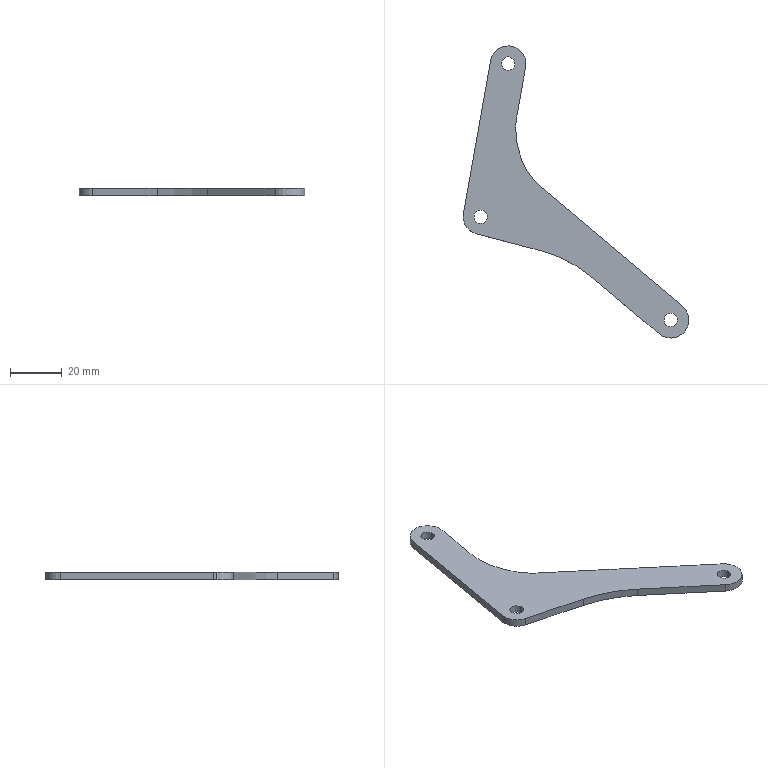Part | SolidWorks | features BaseBody 1 | 1 solid | 20 faces | box 87.081 x 112.72 x 3 mm | volume 7302 mm3 | cylinder 13 | plane 7 | commonest cylinder face diameters 5.2 x6 13.58 x2 62.282 x2 13.715 x1 14 x1 100 x1
STEP:
#1=CARTESIAN_POINT('',(62.068,74.152,3.));
#2=VERTEX_POINT('',#1);
#3=CARTESIAN_POINT('',(56.868,74.152,3.));
#4=VERTEX_POINT('',#3);
#5=CARTESIAN_POINT('',(59.468,74.152,3.));
#6=DIRECTION('',(0.,0.,-1.));
#7=DIRECTION('',(-1.,0.,0.));
#8=AXIS2_PLACEMENT_3D('',#5,#6,#7);
#9=CIRCLE('',#8,2.6);
#10=EDGE_CURVE('',#2,#4,#9,.T.);
#11=ORIENTED_EDGE('',*,*,#10,.F.);
#12=CARTESIAN_POINT('',(62.068,74.152,0.));
#13=VERTEX_POINT('',#12);
#14=CARTESIAN_POINT('',(62.068,74.152,3.));
#15=DIRECTION('',(0.,0.,-1.));
#16=VECTOR('',#15,1000.);
#17=LINE('',#14,#16);
#18=EDGE_CURVE('',#2,#13,#17,.T.);
#19=ORIENTED_EDGE('',*,*,#18,.T.);
#20=CARTESIAN_POINT('',(56.868,74.152,0.));
#21=VERTEX_POINT('',#20);
#22=CARTESIAN_POINT('',(59.468,74.152,0.));
#23=DIRECTION('',(0.,0.,1.));
#24=DIRECTION('',(-1.,0.,0.));
#25=AXIS2_PLACEMENT_3D('',#22,#23,#24);
#26=CIRCLE('',#25,2.6);
#27=EDGE_CURVE('',#21,#13,#26,.T.);
#28=ORIENTED_EDGE('',*,*,#27,.F.);
#29=CARTESIAN_POINT('',(56.868,74.152,3.));
#30=DIRECTION('',(0.,0.,-1.));
#31=VECTOR('',#30,1000.);
#32=LINE('',#29,#31);
#33=EDGE_CURVE('',#4,#21,#32,.T.);
#34=ORIENTED_EDGE('',*,*,#33,.F.);
#35=EDGE_LOOP('',(#11,#19,#28,#34));
#36=FACE_OUTER_BOUND('',#35,.T.);
#37=CARTESIAN_POINT('',(59.468,74.152,3.));
#38=DIRECTION('',(0.,0.,-1.));
#39=DIRECTION('',(-1.,0.,0.));
#40=AXIS2_PLACEMENT_3D('',#37,#38,#39);
#41=CYLINDRICAL_SURFACE('',#40,2.6);
#42=ADVANCED_FACE('',(#36),#41,.F.);
#43=CARTESIAN_POINT('',(62.402,48.808,3.));
#44=VERTEX_POINT('',#43);
#45=CARTESIAN_POINT('',(63.076,55.251,3.));
#46=VERTEX_POINT('',#45);
#47=CARTESIAN_POINT('',(93.543,48.808,3.));
#48=DIRECTION('',(0.,0.,-1.));
#49=DIRECTION('',(-1.,0.,0.));
#50=AXIS2_PLACEMENT_3D('',#47,#48,#49);
#51=CIRCLE('',#50,31.141);
#52=EDGE_CURVE('',#44,#46,#51,.T.);
#53=ORIENTED_EDGE('',*,*,#52,.F.);
#54=CARTESIAN_POINT('',(62.402,48.808,0.));
#55=VERTEX_POINT('',#54);
#56=CARTESIAN_POINT('',(62.402,48.808,3.));
#57=DIRECTION('',(0.,0.,-1.));
#58=VECTOR('',#57,1000.);
#59=LINE('',#56,#58);
#60=EDGE_CURVE('',#44,#55,#59,.T.);
#61=ORIENTED_EDGE('',*,*,#60,.T.);
#62=CARTESIAN_POINT('',(63.076,55.251,0.));
#63=VERTEX_POINT('',#62);
#64=CARTESIAN_POINT('',(93.543,48.808,0.));
#65=DIRECTION('',(0.,0.,1.));
#66=DIRECTION('',(-1.,0.,0.));
#67=AXIS2_PLACEMENT_3D('',#64,#65,#66);
#68=CIRCLE('',#67,31.141);
#69=EDGE_CURVE('',#63,#55,#68,.T.);
#70=ORIENTED_EDGE('',*,*,#69,.F.);
#71=CARTESIAN_POINT('',(63.076,55.251,3.));
#72=DIRECTION('',(0.,0.,-1.));
#73=VECTOR('',#72,1000.);
#74=LINE('',#71,#73);
#75=EDGE_CURVE('',#46,#63,#74,.T.);
#76=ORIENTED_EDGE('',*,*,#75,.F.);
#77=EDGE_LOOP('',(#53,#61,#70,#76));
#78=FACE_OUTER_BOUND('',#77,.T.);
#79=CARTESIAN_POINT('',(93.543,48.808,3.));
#80=DIRECTION('',(0.,0.,-1.));
#81=DIRECTION('',(-1.,0.,0.));
#82=AXIS2_PLACEMENT_3D('',#79,#80,#81);
#83=CYLINDRICAL_SURFACE('',#82,31.141);
#84=ADVANCED_FACE('',(#78),#83,.F.);
#85=CARTESIAN_POINT('',(42.12,15.088,3.));
#86=VERTEX_POINT('',#85);
#87=CARTESIAN_POINT('',(47.182,8.522,3.));
#88=VERTEX_POINT('',#87);
#89=CARTESIAN_POINT('',(48.91,15.088,3.));
#90=DIRECTION('',(0.,0.,1.));
#91=DIRECTION('',(-1.,0.,0.));
#92=AXIS2_PLACEMENT_3D('',#89,#90,#91);
#93=CIRCLE('',#92,6.79);
#94=EDGE_CURVE('',#86,#88,#93,.T.);
#95=ORIENTED_EDGE('',*,*,#94,.F.);
#96=CARTESIAN_POINT('',(42.12,15.088,0.));
#97=VERTEX_POINT('',#96);
#98=CARTESIAN_POINT('',(42.12,15.088,3.));
#99=DIRECTION('',(0.,0.,-1.));
#100=VECTOR('',#99,1000.);
#101=LINE('',#98,#100);
#102=EDGE_CURVE('',#86,#97,#101,.T.);
#103=ORIENTED_EDGE('',*,*,#102,.T.);
#104=CARTESIAN_POINT('',(47.182,8.522,0.));
#105=VERTEX_POINT('',#104);
#106=CARTESIAN_POINT('',(48.91,15.088,0.));
#107=DIRECTION('',(0.,0.,1.));
#108=DIRECTION('',(-1.,0.,0.));
#109=AXIS2_PLACEMENT_3D('',#106,#107,#108);
#110=CIRCLE('',#109,6.79);
#111=EDGE_CURVE('',#97,#105,#110,.T.);
#112=ORIENTED_EDGE('',*,*,#111,.T.);
#113=CARTESIAN_POINT('',(47.182,8.522,3.));
#114=DIRECTION('',(0.,0.,1.));
#115=VECTOR('',#114,1000.);
#116=LINE('',#113,#115);
#117=EDGE_CURVE('',#105,#88,#116,.T.);
#118=ORIENTED_EDGE('',*,*,#117,.T.);
#119=EDGE_LOOP('',(#95,#103,#112,#118));
#120=FACE_OUTER_BOUND('',#119,.T.);
#121=CARTESIAN_POINT('',(48.91,15.088,3.));
#122=DIRECTION('',(0.,0.,-1.));
#123=DIRECTION('',(-1.,0.,0.));
#124=AXIS2_PLACEMENT_3D('',#121,#122,#123);
#125=CYLINDRICAL_SURFACE('',#124,6.79);
#126=ADVANCED_FACE('',(#120),#125,.T.);
#127=CARTESIAN_POINT('',(124.801,-24.711,3.));
#128=VERTEX_POINT('',#127);
#129=CARTESIAN_POINT('',(119.601,-24.711,3.));
#130=VERTEX_POINT('',#129);
#131=CARTESIAN_POINT('',(122.201,-24.711,3.));
#132=DIRECTION('',(0.,0.,-1.));
#133=DIRECTION('',(-1.,0.,0.));
#134=AXIS2_PLACEMENT_3D('',#131,#132,#133);
#135=CIRCLE('',#134,2.6);
#136=EDGE_CURVE('',#128,#130,#135,.T.);
#137=ORIENTED_EDGE('',*,*,#136,.F.);
#138=CARTESIAN_POINT('',(124.801,-24.711,0.));
#139=VERTEX_POINT('',#138);
#140=CARTESIAN_POINT('',(124.801,-24.711,3.));
#141=DIRECTION('',(0.,0.,-1.));
#142=VECTOR('',#141,1000.);
#143=LINE('',#140,#142);
#144=EDGE_CURVE('',#128,#139,#143,.T.);
#145=ORIENTED_EDGE('',*,*,#144,.T.);
#146=CARTESIAN_POINT('',(119.601,-24.711,0.));
#147=VERTEX_POINT('',#146);
#148=CARTESIAN_POINT('',(122.201,-24.711,0.));
#149=DIRECTION('',(0.,0.,1.));
#150=DIRECTION('',(-1.,0.,0.));
#151=AXIS2_PLACEMENT_3D('',#148,#149,#150);
#152=CIRCLE('',#151,2.6);
#153=EDGE_CURVE('',#147,#139,#152,.T.);
#154=ORIENTED_EDGE('',*,*,#153,.F.);
#155=CARTESIAN_POINT('',(119.601,-24.711,3.));
#156=DIRECTION('',(0.,0.,-1.));
#157=VECTOR('',#156,1000.);
#158=LINE('',#155,#157);
#159=EDGE_CURVE('',#130,#147,#158,.T.);
#160=ORIENTED_EDGE('',*,*,#159,.F.);
#161=EDGE_LOOP('',(#137,#145,#154,#160));
#162=FACE_OUTER_BOUND('',#161,.T.);
#163=CARTESIAN_POINT('',(122.201,-24.711,3.));
#164=DIRECTION('',(0.,0.,-1.));
#165=DIRECTION('',(-1.,0.,0.));
#166=AXIS2_PLACEMENT_3D('',#163,#164,#165);
#167=CYLINDRICAL_SURFACE('',#166,2.6);
#168=ADVANCED_FACE('',(#162),#167,.F.);
#169=CARTESIAN_POINT('',(51.51,15.088,3.));
#170=VERTEX_POINT('',#169);
#171=CARTESIAN_POINT('',(46.31,15.088,3.));
#172=VERTEX_POINT('',#171);
#173=CARTESIAN_POINT('',(48.91,15.088,3.));
#174=DIRECTION('',(0.,0.,-1.));
#175=DIRECTION('',(-1.,0.,0.));
#176=AXIS2_PLACEMENT_3D('',#173,#174,#175);
#177=CIRCLE('',#176,2.6);
#178=EDGE_CURVE('',#170,#172,#177,.T.);
#179=ORIENTED_EDGE('',*,*,#178,.F.);
#180=CARTESIAN_POINT('',(51.51,15.088,0.));
#181=VERTEX_POINT('',#180);
#182=CARTESIAN_POINT('',(51.51,15.088,3.));
#183=DIRECTION('',(0.,0.,-1.));
#184=VECTOR('',#183,1000.);
#185=LINE('',#182,#184);
#186=EDGE_CURVE('',#170,#181,#185,.T.);
#187=ORIENTED_EDGE('',*,*,#186,.T.);
#188=CARTESIAN_POINT('',(46.31,15.088,0.));
#189=VERTEX_POINT('',#188);
#190=CARTESIAN_POINT('',(48.91,15.088,0.));
#191=DIRECTION('',(0.,0.,1.));
#192=DIRECTION('',(-1.,0.,0.));
#193=AXIS2_PLACEMENT_3D('',#190,#191,#192);
#194=CIRCLE('',#193,2.6);
#195=EDGE_CURVE('',#189,#181,#194,.T.);
#196=ORIENTED_EDGE('',*,*,#195,.F.);
#197=CARTESIAN_POINT('',(46.31,15.088,3.));
#198=DIRECTION('',(0.,0.,-1.));
#199=VECTOR('',#198,1000.);
#200=LINE('',#197,#199);
#201=EDGE_CURVE('',#172,#189,#200,.T.);
#202=ORIENTED_EDGE('',*,*,#201,.F.);
#203=EDGE_LOOP('',(#179,#187,#196,#202));
#204=FACE_OUTER_BOUND('',#203,.T.);
#205=CARTESIAN_POINT('',(48.91,15.088,3.));
#206=DIRECTION('',(0.,0.,-1.));
#207=DIRECTION('',(-1.,0.,0.));
#208=AXIS2_PLACEMENT_3D('',#205,#206,#207);
#209=CYLINDRICAL_SURFACE('',#208,2.6);
#210=ADVANCED_FACE('',(#204),#209,.F.);
#211=CARTESIAN_POINT('',(59.468,74.152,3.));
#212=DIRECTION('',(0.,0.,-1.));
#213=DIRECTION('',(-1.,0.,0.));
#214=AXIS2_PLACEMENT_3D('',#211,#212,#213);
#215=CIRCLE('',#214,2.6);
#216=EDGE_CURVE('',#4,#2,#215,.T.);
#217=ORIENTED_EDGE('',*,*,#216,.T.);
#218=ORIENTED_EDGE('',*,*,#10,.T.);
#219=EDGE_LOOP('',(#217,#218));
#220=FACE_BOUND('',#219,.T.);
#221=CARTESIAN_POINT('',(70.256,28.133,3.));
#222=VERTEX_POINT('',#221);
#223=CARTESIAN_POINT('',(93.543,48.808,3.));
#224=DIRECTION('',(0.,0.,-1.));
#225=DIRECTION('',(-1.,0.,0.));
#226=AXIS2_PLACEMENT_3D('',#223,#224,#225);
#227=CIRCLE('',#226,31.141);
#228=EDGE_CURVE('',#222,#44,#227,.T.);
#229=ORIENTED_EDGE('',*,*,#228,.T.);
#230=ORIENTED_EDGE('',*,*,#52,.T.);
#231=CARTESIAN_POINT('',(66.219,72.953,3.));
#232=VERTEX_POINT('',#231);
#233=CARTESIAN_POINT('',(63.076,55.251,3.));
#234=DIRECTION('',(0.1749,0.9846,0.));
#235=VECTOR('',#234,1000.);
#236=LINE('',#233,#235);
#237=EDGE_CURVE('',#46,#232,#236,.T.);
#238=ORIENTED_EDGE('',*,*,#237,.T.);
#239=CARTESIAN_POINT('',(52.716,75.351,3.));
#240=VERTEX_POINT('',#239);
#241=CARTESIAN_POINT('',(59.468,74.152,3.));
#242=DIRECTION('',(0.,0.,1.));
#243=DIRECTION('',(-1.,0.,0.));
#244=AXIS2_PLACEMENT_3D('',#241,#242,#243);
#245=CIRCLE('',#244,6.857);
#246=EDGE_CURVE('',#232,#240,#245,.T.);
#247=ORIENTED_EDGE('',*,*,#246,.T.);
#248=CARTESIAN_POINT('',(42.225,16.276,3.));
#249=VERTEX_POINT('',#248);
#250=CARTESIAN_POINT('',(52.716,75.351,3.));
#251=DIRECTION('',(-0.1749,-0.9846,0.));
#252=VECTOR('',#251,1000.);
#253=LINE('',#250,#252);
#254=EDGE_CURVE('',#240,#249,#253,.T.);
#255=ORIENTED_EDGE('',*,*,#254,.T.);
#256=CARTESIAN_POINT('',(48.91,15.088,3.));
#257=DIRECTION('',(0.,0.,1.));
#258=DIRECTION('',(-1.,0.,0.));
#259=AXIS2_PLACEMENT_3D('',#256,#257,#258);
#260=CIRCLE('',#259,6.79);
#261=EDGE_CURVE('',#249,#86,#260,.T.);
#262=ORIENTED_EDGE('',*,*,#261,.T.);
#263=ORIENTED_EDGE('',*,*,#94,.T.);
#264=CARTESIAN_POINT('',(72.182,1.941,3.));
#265=VERTEX_POINT('',#264);
#266=CARTESIAN_POINT('',(47.182,8.522,3.));
#267=DIRECTION('',(0.9671,-0.2546,0.));
#268=VECTOR('',#267,1000.);
#269=LINE('',#266,#268);
#270=EDGE_CURVE('',#88,#265,#269,.T.);
#271=ORIENTED_EDGE('',*,*,#270,.T.);
#272=CARTESIAN_POINT('',(91.639,-8.149,3.));
#273=VERTEX_POINT('',#272);
#274=CARTESIAN_POINT('',(59.453,-46.412,3.));
#275=DIRECTION('',(0.,0.,-1.));
#276=DIRECTION('',(-1.,0.,0.));
#277=AXIS2_PLACEMENT_3D('',#274,#275,#276);
#278=CIRCLE('',#277,50.);
#279=EDGE_CURVE('',#265,#273,#278,.T.);
#280=ORIENTED_EDGE('',*,*,#279,.T.);
#281=CARTESIAN_POINT('',(117.695,-30.067,3.));
#282=VERTEX_POINT('',#281);
#283=CARTESIAN_POINT('',(91.639,-8.149,3.));
#284=DIRECTION('',(0.7653,-0.6437,0.));
#285=VECTOR('',#284,1000.);
#286=LINE('',#283,#285);
#287=EDGE_CURVE('',#273,#282,#286,.T.);
#288=ORIENTED_EDGE('',*,*,#287,.T.);
#289=CARTESIAN_POINT('',(126.707,-19.354,3.));
#290=VERTEX_POINT('',#289);
#291=CARTESIAN_POINT('',(122.201,-24.711,3.));
#292=DIRECTION('',(0.,0.,1.));
#293=DIRECTION('',(-1.,0.,0.));
#294=AXIS2_PLACEMENT_3D('',#291,#292,#293);
#295=CIRCLE('',#294,7.);
#296=EDGE_CURVE('',#282,#290,#295,.T.);
#297=ORIENTED_EDGE('',*,*,#296,.T.);
#298=CARTESIAN_POINT('',(126.707,-19.354,3.));
#299=DIRECTION('',(-0.7653,0.6437,0.));
#300=VECTOR('',#299,1000.);
#301=LINE('',#298,#300);
#302=EDGE_CURVE('',#290,#222,#301,.T.);
#303=ORIENTED_EDGE('',*,*,#302,.T.);
#304=EDGE_LOOP('',(#229,#230,#238,#247,#255,#262,#263,#271,#280,#288,#297,#303));
#305=FACE_OUTER_BOUND('',#304,.T.);
#306=CARTESIAN_POINT('',(122.201,-24.711,3.));
#307=DIRECTION('',(0.,0.,-1.));
#308=DIRECTION('',(-1.,0.,0.));
#309=AXIS2_PLACEMENT_3D('',#306,#307,#308);
#310=CIRCLE('',#309,2.6);
#311=EDGE_CURVE('',#130,#128,#310,.T.);
#312=ORIENTED_EDGE('',*,*,#311,.T.);
#313=ORIENTED_EDGE('',*,*,#136,.T.);
#314=EDGE_LOOP('',(#312,#313));
#315=FACE_BOUND('',#314,.T.);
#316=CARTESIAN_POINT('',(48.91,15.088,3.));
#317=DIRECTION('',(0.,0.,-1.));
#318=DIRECTION('',(-1.,0.,0.));
#319=AXIS2_PLACEMENT_3D('',#316,#317,#318);
#320=CIRCLE('',#319,2.6);
#321=EDGE_CURVE('',#172,#170,#320,.T.);
#322=ORIENTED_EDGE('',*,*,#321,.T.);
#323=ORIENTED_EDGE('',*,*,#178,.T.);
#324=EDGE_LOOP('',(#322,#323));
#325=FACE_BOUND('',#324,.T.);
#326=CARTESIAN_POINT('',(48.91,15.088,3.));
#327=DIRECTION('',(0.,0.,1.));
#328=DIRECTION('',(1.,0.,0.));
#329=AXIS2_PLACEMENT_3D('',#326,#327,#328);
#330=PLANE('',#329);
#331=ADVANCED_FACE('',(#220,#305,#315,#325),#330,.T.);
#332=ORIENTED_EDGE('',*,*,#18,.F.);
#333=ORIENTED_EDGE('',*,*,#216,.F.);
#334=ORIENTED_EDGE('',*,*,#33,.T.);
#335=CARTESIAN_POINT('',(59.468,74.152,0.));
#336=DIRECTION('',(0.,0.,1.));
#337=DIRECTION('',(-1.,0.,0.));
#338=AXIS2_PLACEMENT_3D('',#335,#336,#337);
#339=CIRCLE('',#338,2.6);
#340=EDGE_CURVE('',#13,#21,#339,.T.);
#341=ORIENTED_EDGE('',*,*,#340,.F.);
#342=EDGE_LOOP('',(#332,#333,#334,#341));
#343=FACE_OUTER_BOUND('',#342,.T.);
#344=CARTESIAN_POINT('',(59.468,74.152,3.));
#345=DIRECTION('',(0.,0.,-1.));
#346=DIRECTION('',(-1.,0.,0.));
#347=AXIS2_PLACEMENT_3D('',#344,#345,#346);
#348=CYLINDRICAL_SURFACE('',#347,2.6);
#349=ADVANCED_FACE('',(#343),#348,.F.);
#350=ORIENTED_EDGE('',*,*,#60,.F.);
#351=ORIENTED_EDGE('',*,*,#228,.F.);
#352=CARTESIAN_POINT('',(70.256,28.133,0.));
#353=VERTEX_POINT('',#352);
#354=CARTESIAN_POINT('',(70.256,28.133,3.));
#355=DIRECTION('',(0.,0.,1.));
#356=VECTOR('',#355,1000.);
#357=LINE('',#354,#356);
#358=EDGE_CURVE('',#353,#222,#357,.T.);
#359=ORIENTED_EDGE('',*,*,#358,.F.);
#360=CARTESIAN_POINT('',(93.543,48.808,0.));
#361=DIRECTION('',(0.,0.,1.));
#362=DIRECTION('',(-1.,0.,0.));
#363=AXIS2_PLACEMENT_3D('',#360,#361,#362);
#364=CIRCLE('',#363,31.141);
#365=EDGE_CURVE('',#55,#353,#364,.T.);
#366=ORIENTED_EDGE('',*,*,#365,.F.);
#367=EDGE_LOOP('',(#350,#351,#359,#366));
#368=FACE_OUTER_BOUND('',#367,.T.);
#369=CARTESIAN_POINT('',(93.543,48.808,3.));
#370=DIRECTION('',(0.,0.,-1.));
#371=DIRECTION('',(-1.,0.,0.));
#372=AXIS2_PLACEMENT_3D('',#369,#370,#371);
#373=CYLINDRICAL_SURFACE('',#372,31.141);
#374=ADVANCED_FACE('',(#368),#373,.F.);
#375=ORIENTED_EDGE('',*,*,#302,.F.);
#376=CARTESIAN_POINT('',(126.707,-19.354,0.));
#377=VERTEX_POINT('',#376);
#378=CARTESIAN_POINT('',(126.707,-19.354,3.));
#379=DIRECTION('',(0.,0.,1.));
#380=VECTOR('',#379,1000.);
#381=LINE('',#378,#380);
#382=EDGE_CURVE('',#377,#290,#381,.T.);
#383=ORIENTED_EDGE('',*,*,#382,.F.);
#384=CARTESIAN_POINT('',(70.256,28.133,0.));
#385=DIRECTION('',(0.7653,-0.6437,0.));
#386=VECTOR('',#385,1000.);
#387=LINE('',#384,#386);
#388=EDGE_CURVE('',#353,#377,#387,.T.);
#389=ORIENTED_EDGE('',*,*,#388,.F.);
#390=ORIENTED_EDGE('',*,*,#358,.T.);
#391=EDGE_LOOP('',(#375,#383,#389,#390));
#392=FACE_OUTER_BOUND('',#391,.T.);
#393=CARTESIAN_POINT('',(70.256,28.133,3.));
#394=DIRECTION('',(-0.6437,-0.7653,0.));
#395=DIRECTION('',(0.7653,-0.6437,0.));
#396=AXIS2_PLACEMENT_3D('',#393,#394,#395);
#397=PLANE('',#396);
#398=ADVANCED_FACE('',(#392),#397,.F.);
#399=CARTESIAN_POINT('',(117.695,-30.067,0.));
#400=VERTEX_POINT('',#399);
#401=CARTESIAN_POINT('',(122.201,-24.711,0.));
#402=DIRECTION('',(0.,0.,1.));
#403=DIRECTION('',(-1.,0.,0.));
#404=AXIS2_PLACEMENT_3D('',#401,#402,#403);
#405=CIRCLE('',#404,7.);
#406=EDGE_CURVE('',#400,#377,#405,.T.);
#407=ORIENTED_EDGE('',*,*,#406,.T.);
#408=ORIENTED_EDGE('',*,*,#382,.T.);
#409=ORIENTED_EDGE('',*,*,#296,.F.);
#410=CARTESIAN_POINT('',(117.695,-30.067,3.));
#411=DIRECTION('',(0.,0.,-1.));
#412=VECTOR('',#411,1000.);
#413=LINE('',#410,#412);
#414=EDGE_CURVE('',#282,#400,#413,.T.);
#415=ORIENTED_EDGE('',*,*,#414,.T.);
#416=EDGE_LOOP('',(#407,#408,#409,#415));
#417=FACE_OUTER_BOUND('',#416,.T.);
#418=CARTESIAN_POINT('',(122.201,-24.711,3.));
#419=DIRECTION('',(0.,0.,-1.));
#420=DIRECTION('',(-1.,0.,0.));
#421=AXIS2_PLACEMENT_3D('',#418,#419,#420);
#422=CYLINDRICAL_SURFACE('',#421,7.);
#423=ADVANCED_FACE('',(#417),#422,.T.);
#424=ORIENTED_EDGE('',*,*,#287,.F.);
#425=CARTESIAN_POINT('',(91.639,-8.149,0.));
#426=VERTEX_POINT('',#425);
#427=CARTESIAN_POINT('',(91.639,-8.149,3.));
#428=DIRECTION('',(0.,0.,1.));
#429=VECTOR('',#428,1000.);
#430=LINE('',#427,#429);
#431=EDGE_CURVE('',#426,#273,#430,.T.);
#432=ORIENTED_EDGE('',*,*,#431,.F.);
#433=CARTESIAN_POINT('',(117.695,-30.067,0.));
#434=DIRECTION('',(-0.7653,0.6437,0.));
#435=VECTOR('',#434,1000.);
#436=LINE('',#433,#435);
#437=EDGE_CURVE('',#400,#426,#436,.T.);
#438=ORIENTED_EDGE('',*,*,#437,.F.);
#439=ORIENTED_EDGE('',*,*,#414,.F.);
#440=EDGE_LOOP('',(#424,#432,#438,#439));
#441=FACE_OUTER_BOUND('',#440,.T.);
#442=CARTESIAN_POINT('',(117.695,-30.067,3.));
#443=DIRECTION('',(0.6437,0.7653,0.));
#444=DIRECTION('',(-0.7653,0.6437,0.));
#445=AXIS2_PLACEMENT_3D('',#442,#443,#444);
#446=PLANE('',#445);
#447=ADVANCED_FACE('',(#441),#446,.F.);
#448=ORIENTED_EDGE('',*,*,#279,.F.);
#449=CARTESIAN_POINT('',(72.182,1.941,0.));
#450=VERTEX_POINT('',#449);
#451=CARTESIAN_POINT('',(72.182,1.941,3.));
#452=DIRECTION('',(0.,0.,1.));
#453=VECTOR('',#452,1000.);
#454=LINE('',#451,#453);
#455=EDGE_CURVE('',#450,#265,#454,.T.);
#456=ORIENTED_EDGE('',*,*,#455,.F.);
#457=CARTESIAN_POINT('',(59.453,-46.412,0.));
#458=DIRECTION('',(0.,0.,1.));
#459=DIRECTION('',(-1.,0.,0.));
#460=AXIS2_PLACEMENT_3D('',#457,#458,#459);
#461=CIRCLE('',#460,50.);
#462=EDGE_CURVE('',#426,#450,#461,.T.);
#463=ORIENTED_EDGE('',*,*,#462,.F.);
#464=ORIENTED_EDGE('',*,*,#431,.T.);
#465=EDGE_LOOP('',(#448,#456,#463,#464));
#466=FACE_OUTER_BOUND('',#465,.T.);
#467=CARTESIAN_POINT('',(59.453,-46.412,3.));
#468=DIRECTION('',(0.,0.,-1.));
#469=DIRECTION('',(-1.,0.,0.));
#470=AXIS2_PLACEMENT_3D('',#467,#468,#469);
#471=CYLINDRICAL_SURFACE('',#470,50.);
#472=ADVANCED_FACE('',(#466),#471,.F.);
#473=ORIENTED_EDGE('',*,*,#270,.F.);
#474=ORIENTED_EDGE('',*,*,#117,.F.);
#475=CARTESIAN_POINT('',(72.182,1.941,0.));
#476=DIRECTION('',(-0.9671,0.2546,0.));
#477=VECTOR('',#476,1000.);
#478=LINE('',#475,#477);
#479=EDGE_CURVE('',#450,#105,#478,.T.);
#480=ORIENTED_EDGE('',*,*,#479,.F.);
#481=ORIENTED_EDGE('',*,*,#455,.T.);
#482=EDGE_LOOP('',(#473,#474,#480,#481));
#483=FACE_OUTER_BOUND('',#482,.T.);
#484=CARTESIAN_POINT('',(72.182,1.941,3.));
#485=DIRECTION('',(0.2546,0.9671,0.));
#486=DIRECTION('',(-0.9671,0.2546,0.));
#487=AXIS2_PLACEMENT_3D('',#484,#485,#486);
#488=PLANE('',#487);
#489=ADVANCED_FACE('',(#483),#488,.F.);
#490=ORIENTED_EDGE('',*,*,#102,.F.);
#491=ORIENTED_EDGE('',*,*,#261,.F.);
#492=CARTESIAN_POINT('',(42.225,16.276,0.));
#493=VERTEX_POINT('',#492);
#494=CARTESIAN_POINT('',(42.225,16.276,3.));
#495=DIRECTION('',(0.,0.,-1.));
#496=VECTOR('',#495,1000.);
#497=LINE('',#494,#496);
#498=EDGE_CURVE('',#249,#493,#497,.T.);
#499=ORIENTED_EDGE('',*,*,#498,.T.);
#500=CARTESIAN_POINT('',(48.91,15.088,0.));
#501=DIRECTION('',(0.,0.,1.));
#502=DIRECTION('',(-1.,0.,0.));
#503=AXIS2_PLACEMENT_3D('',#500,#501,#502);
#504=CIRCLE('',#503,6.79);
#505=EDGE_CURVE('',#493,#97,#504,.T.);
#506=ORIENTED_EDGE('',*,*,#505,.T.);
#507=EDGE_LOOP('',(#490,#491,#499,#506));
#508=FACE_OUTER_BOUND('',#507,.T.);
#509=CARTESIAN_POINT('',(48.91,15.088,3.));
#510=DIRECTION('',(0.,0.,-1.));
#511=DIRECTION('',(-1.,0.,0.));
#512=AXIS2_PLACEMENT_3D('',#509,#510,#511);
#513=CYLINDRICAL_SURFACE('',#512,6.79);
#514=ADVANCED_FACE('',(#508),#513,.T.);
#515=ORIENTED_EDGE('',*,*,#254,.F.);
#516=CARTESIAN_POINT('',(52.716,75.351,0.));
#517=VERTEX_POINT('',#516);
#518=CARTESIAN_POINT('',(52.716,75.351,3.));
#519=DIRECTION('',(0.,0.,1.));
#520=VECTOR('',#519,1000.);
#521=LINE('',#518,#520);
#522=EDGE_CURVE('',#517,#240,#521,.T.);
#523=ORIENTED_EDGE('',*,*,#522,.F.);
#524=CARTESIAN_POINT('',(46.025,37.673,0.));
#525=DIRECTION('',(0.1749,0.9846,0.));
#526=VECTOR('',#525,1000.);
#527=LINE('',#524,#526);
#528=EDGE_CURVE('',#493,#517,#527,.T.);
#529=ORIENTED_EDGE('',*,*,#528,.F.);
#530=ORIENTED_EDGE('',*,*,#498,.F.);
#531=EDGE_LOOP('',(#515,#523,#529,#530));
#532=FACE_OUTER_BOUND('',#531,.T.);
#533=CARTESIAN_POINT('',(46.025,37.673,3.));
#534=DIRECTION('',(0.9846,-0.1749,0.));
#535=DIRECTION('',(0.1749,0.9846,0.));
#536=AXIS2_PLACEMENT_3D('',#533,#534,#535);
#537=PLANE('',#536);
#538=ADVANCED_FACE('',(#532),#537,.F.);
#539=CARTESIAN_POINT('',(66.219,72.953,0.));
#540=VERTEX_POINT('',#539);
#541=CARTESIAN_POINT('',(59.468,74.152,0.));
#542=DIRECTION('',(0.,0.,1.));
#543=DIRECTION('',(-1.,0.,0.));
#544=AXIS2_PLACEMENT_3D('',#541,#542,#543);
#545=CIRCLE('',#544,6.857);
#546=EDGE_CURVE('',#540,#517,#545,.T.);
#547=ORIENTED_EDGE('',*,*,#546,.T.);
#548=ORIENTED_EDGE('',*,*,#522,.T.);
#549=ORIENTED_EDGE('',*,*,#246,.F.);
#550=CARTESIAN_POINT('',(66.219,72.953,3.));
#551=DIRECTION('',(0.,0.,-1.));
#552=VECTOR('',#551,1000.);
#553=LINE('',#550,#552);
#554=EDGE_CURVE('',#232,#540,#553,.T.);
#555=ORIENTED_EDGE('',*,*,#554,.T.);
#556=EDGE_LOOP('',(#547,#548,#549,#555));
#557=FACE_OUTER_BOUND('',#556,.T.);
#558=CARTESIAN_POINT('',(59.468,74.152,3.));
#559=DIRECTION('',(0.,0.,-1.));
#560=DIRECTION('',(-1.,0.,0.));
#561=AXIS2_PLACEMENT_3D('',#558,#559,#560);
#562=CYLINDRICAL_SURFACE('',#561,6.857);
#563=ADVANCED_FACE('',(#557),#562,.T.);
#564=ORIENTED_EDGE('',*,*,#237,.F.);
#565=ORIENTED_EDGE('',*,*,#75,.T.);
#566=CARTESIAN_POINT('',(66.219,72.953,0.));
#567=DIRECTION('',(-0.1749,-0.9846,0.));
#568=VECTOR('',#567,1000.);
#569=LINE('',#566,#568);
#570=EDGE_CURVE('',#540,#63,#569,.T.);
#571=ORIENTED_EDGE('',*,*,#570,.F.);
#572=ORIENTED_EDGE('',*,*,#554,.F.);
#573=EDGE_LOOP('',(#564,#565,#571,#572));
#574=FACE_OUTER_BOUND('',#573,.T.);
#575=CARTESIAN_POINT('',(66.219,72.953,3.));
#576=DIRECTION('',(-0.9846,0.1749,0.));
#577=DIRECTION('',(-0.1749,-0.9846,0.));
#578=AXIS2_PLACEMENT_3D('',#575,#576,#577);
#579=PLANE('',#578);
#580=ADVANCED_FACE('',(#574),#579,.F.);
#581=ORIENTED_EDGE('',*,*,#144,.F.);
#582=ORIENTED_EDGE('',*,*,#311,.F.);
#583=ORIENTED_EDGE('',*,*,#159,.T.);
#584=CARTESIAN_POINT('',(122.201,-24.711,0.));
#585=DIRECTION('',(0.,0.,1.));
#586=DIRECTION('',(-1.,0.,0.));
#587=AXIS2_PLACEMENT_3D('',#584,#585,#586);
#588=CIRCLE('',#587,2.6);
#589=EDGE_CURVE('',#139,#147,#588,.T.);
#590=ORIENTED_EDGE('',*,*,#589,.F.);
#591=EDGE_LOOP('',(#581,#582,#583,#590));
#592=FACE_OUTER_BOUND('',#591,.T.);
#593=CARTESIAN_POINT('',(122.201,-24.711,3.));
#594=DIRECTION('',(0.,0.,-1.));
#595=DIRECTION('',(-1.,0.,0.));
#596=AXIS2_PLACEMENT_3D('',#593,#594,#595);
#597=CYLINDRICAL_SURFACE('',#596,2.6);
#598=ADVANCED_FACE('',(#592),#597,.F.);
#599=ORIENTED_EDGE('',*,*,#186,.F.);
#600=ORIENTED_EDGE('',*,*,#321,.F.);
#601=ORIENTED_EDGE('',*,*,#201,.T.);
#602=CARTESIAN_POINT('',(48.91,15.088,0.));
#603=DIRECTION('',(0.,0.,1.));
#604=DIRECTION('',(-1.,0.,0.));
#605=AXIS2_PLACEMENT_3D('',#602,#603,#604);
#606=CIRCLE('',#605,2.6);
#607=EDGE_CURVE('',#181,#189,#606,.T.);
#608=ORIENTED_EDGE('',*,*,#607,.F.);
#609=EDGE_LOOP('',(#599,#600,#601,#608));
#610=FACE_OUTER_BOUND('',#609,.T.);
#611=CARTESIAN_POINT('',(48.91,15.088,3.));
#612=DIRECTION('',(0.,0.,-1.));
#613=DIRECTION('',(-1.,0.,0.));
#614=AXIS2_PLACEMENT_3D('',#611,#612,#613);
#615=CYLINDRICAL_SURFACE('',#614,2.6);
#616=ADVANCED_FACE('',(#610),#615,.F.);
#617=ORIENTED_EDGE('',*,*,#546,.F.);
#618=ORIENTED_EDGE('',*,*,#570,.T.);
#619=ORIENTED_EDGE('',*,*,#69,.T.);
#620=ORIENTED_EDGE('',*,*,#365,.T.);
#621=ORIENTED_EDGE('',*,*,#388,.T.);
#622=ORIENTED_EDGE('',*,*,#406,.F.);
#623=ORIENTED_EDGE('',*,*,#437,.T.);
#624=ORIENTED_EDGE('',*,*,#462,.T.);
#625=ORIENTED_EDGE('',*,*,#479,.T.);
#626=ORIENTED_EDGE('',*,*,#111,.F.);
#627=ORIENTED_EDGE('',*,*,#505,.F.);
#628=ORIENTED_EDGE('',*,*,#528,.T.);
#629=EDGE_LOOP('',(#617,#618,#619,#620,#621,#622,#623,#624,#625,#626,#627,#628));
#630=FACE_OUTER_BOUND('',#629,.T.);
#631=ORIENTED_EDGE('',*,*,#153,.T.);
#632=ORIENTED_EDGE('',*,*,#589,.T.);
#633=EDGE_LOOP('',(#631,#632));
#634=FACE_BOUND('',#633,.T.);
#635=ORIENTED_EDGE('',*,*,#27,.T.);
#636=ORIENTED_EDGE('',*,*,#340,.T.);
#637=EDGE_LOOP('',(#635,#636));
#638=FACE_BOUND('',#637,.T.);
#639=ORIENTED_EDGE('',*,*,#195,.T.);
#640=ORIENTED_EDGE('',*,*,#607,.T.);
#641=EDGE_LOOP('',(#639,#640));
#642=FACE_BOUND('',#641,.T.);
#643=CARTESIAN_POINT('',(48.91,15.088,0.));
#644=DIRECTION('',(0.,0.,1.));
#645=DIRECTION('',(1.,0.,0.));
#646=AXIS2_PLACEMENT_3D('',#643,#644,#645);
#647=PLANE('',#646);
#648=ADVANCED_FACE('',(#630,#634,#638,#642),#647,.F.);
#649=CLOSED_SHELL('',(#42,#84,#126,#168,#210,#331,#349,#374,#398,#423,#447,#472,#489,#514,#538,#563,#580,#598,#616,#648));
#650=MANIFOLD_SOLID_BREP('',#649);
#651=CARTESIAN_POINT('',(0.,0.,0.));
#652=DIRECTION('',(0.,0.,1.));
#653=DIRECTION('',(1.,0.,0.));
#654=AXIS2_PLACEMENT_3D('',#651,#652,#653);
#655=(LENGTH_UNIT()NAMED_UNIT(*)SI_UNIT(.MILLI.,.METRE.));
#656=UNCERTAINTY_MEASURE_WITH_UNIT(LENGTH_MEASURE(0.00001),#655,'','');
#657=(NAMED_UNIT(*)PLANE_ANGLE_UNIT()SI_UNIT($,.RADIAN.));
#658=(NAMED_UNIT(*)SI_UNIT($,.STERADIAN.)SOLID_ANGLE_UNIT());
#659=(GEOMETRIC_REPRESENTATION_CONTEXT(3)GLOBAL_UNCERTAINTY_ASSIGNED_CONTEXT((#656))GLOBAL_UNIT_ASSIGNED_CONTEXT((#655,#657,#658))REPRESENTATION_CONTEXT('',''));
#660=ADVANCED_BREP_SHAPE_REPRESENTATION('',(#650,#654),#659);